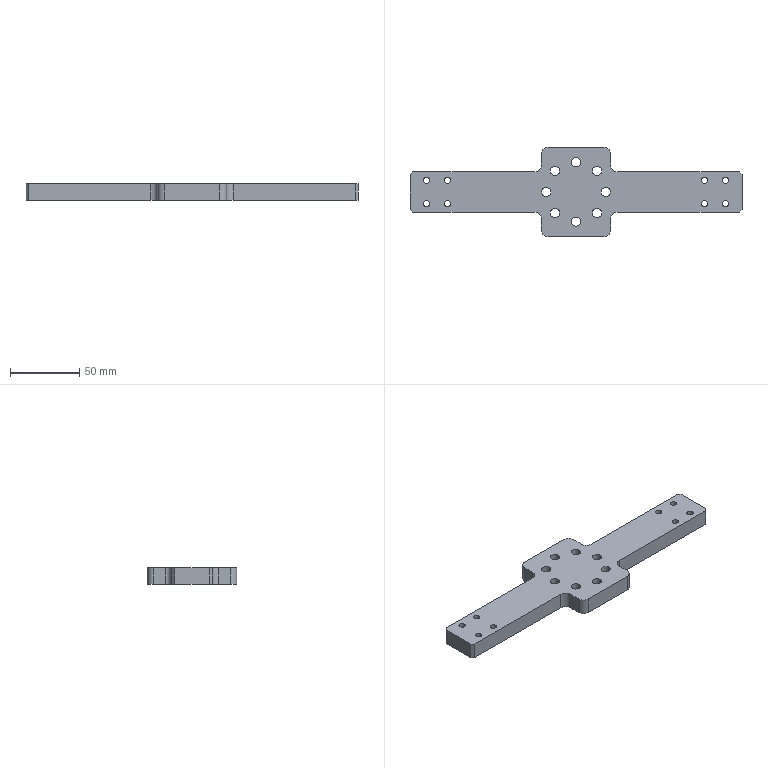Part | SolidWorks | features HoleWzd 2, Chamfer 1, Extrusion 1, Fillet 1, ICE 1, MirrorPattern 1 | 1 solid | 82 faces | box 240 x 65 x 12 mm | volume 96904 mm3 | cylinder 56 | plane 26 | commonest cylinder face diameters 4.5 x16 6.6 x16 11 x16 10 x8